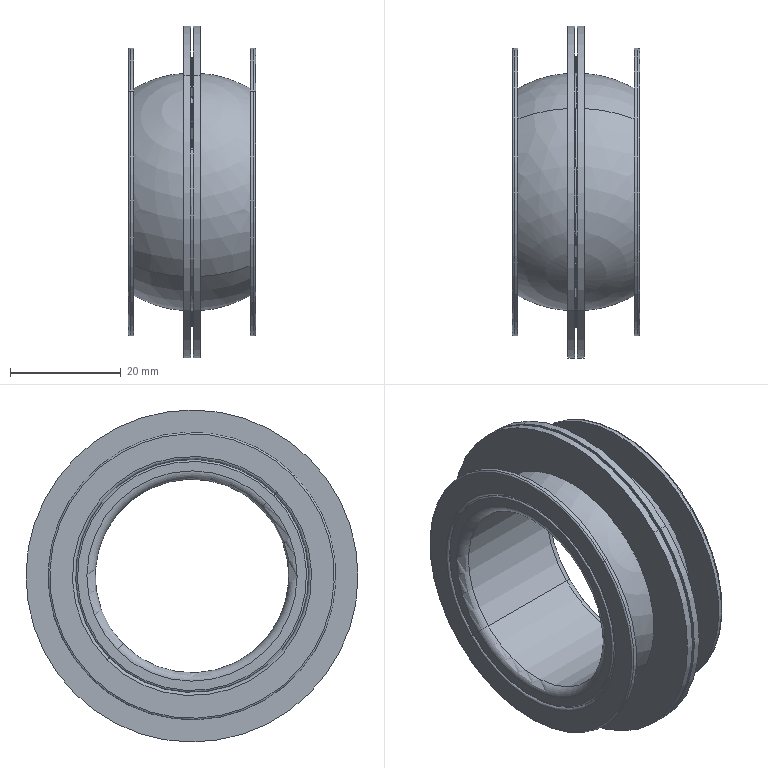Part | SolidWorks | features BaseBody 1 | 1 solid | 56 faces | volume 13898 mm3 | cylinder 18 | torus 16 | plane 12 | sphere 10 | commonest cylinder face diameters 42 x4 42.2 x4 52 x4 60 x4 35 x2
STEP:
#1=CARTESIAN_POINT('',(249.,13.531,-13.338));
#2=VERTEX_POINT('',#1);
#3=CARTESIAN_POINT('',(249.,-13.531,13.338));
#4=VERTEX_POINT('',#3);
#5=CARTESIAN_POINT('',(249.,0.,0.));
#6=DIRECTION('',(1.,0.,0.));
#7=DIRECTION('',(0.,-0.7122,0.702));
#8=AXIS2_PLACEMENT_3D('',#5,#6,#7);
#9=CIRCLE('',#8,19.);
#10=EDGE_CURVE('',#2,#4,#9,.T.);
#11=ORIENTED_EDGE('',*,*,#10,.F.);
#12=CARTESIAN_POINT('',(250.5,12.463,-12.285));
#13=VERTEX_POINT('',#12);
#14=CARTESIAN_POINT('',(250.5,13.531,-13.338));
#15=DIRECTION('',(0.,0.702,0.7122));
#16=DIRECTION('',(0.,-0.7122,0.702));
#17=AXIS2_PLACEMENT_3D('',#14,#15,#16);
#18=CIRCLE('',#17,1.5);
#19=EDGE_CURVE('',#2,#13,#18,.T.);
#20=ORIENTED_EDGE('',*,*,#19,.T.);
#21=CARTESIAN_POINT('',(250.5,-12.463,12.285));
#22=VERTEX_POINT('',#21);
#23=CARTESIAN_POINT('',(250.5,0.,0.));
#24=DIRECTION('',(-1.,0.,0.));
#25=DIRECTION('',(0.,-0.7122,0.702));
#26=AXIS2_PLACEMENT_3D('',#23,#24,#25);
#27=CIRCLE('',#26,17.5);
#28=EDGE_CURVE('',#22,#13,#27,.T.);
#29=ORIENTED_EDGE('',*,*,#28,.F.);
#30=CARTESIAN_POINT('',(250.5,-13.531,13.338));
#31=DIRECTION('',(0.,-0.702,-0.7122));
#32=DIRECTION('',(0.,0.7122,-0.702));
#33=AXIS2_PLACEMENT_3D('',#30,#31,#32);
#34=CIRCLE('',#33,1.5);
#35=EDGE_CURVE('',#4,#22,#34,.T.);
#36=ORIENTED_EDGE('',*,*,#35,.F.);
#37=EDGE_LOOP('',(#11,#20,#29,#36));
#38=FACE_OUTER_BOUND('',#37,.T.);
#39=CARTESIAN_POINT('',(250.5,0.,0.));
#40=DIRECTION('',(-1.,0.,0.));
#41=DIRECTION('',(0.,-0.7122,0.702));
#42=AXIS2_PLACEMENT_3D('',#39,#40,#41);
#43=TOROIDAL_SURFACE('',#42,19.,1.5);
#44=ADVANCED_FACE('',(#38),#43,.T.);
#45=CARTESIAN_POINT('',(272.,-13.531,13.338));
#46=VERTEX_POINT('',#45);
#47=CARTESIAN_POINT('',(272.,13.531,-13.338));
#48=VERTEX_POINT('',#47);
#49=CARTESIAN_POINT('',(272.,0.,0.));
#50=DIRECTION('',(-1.,0.,0.));
#51=DIRECTION('',(0.,0.7122,-0.702));
#52=AXIS2_PLACEMENT_3D('',#49,#50,#51);
#53=CIRCLE('',#52,19.);
#54=EDGE_CURVE('',#46,#48,#53,.T.);
#55=ORIENTED_EDGE('',*,*,#54,.F.);
#56=CARTESIAN_POINT('',(270.5,-12.463,12.285));
#57=VERTEX_POINT('',#56);
#58=CARTESIAN_POINT('',(270.5,-13.531,13.338));
#59=DIRECTION('',(0.,0.702,0.7122));
#60=DIRECTION('',(0.,-0.7122,0.702));
#61=AXIS2_PLACEMENT_3D('',#58,#59,#60);
#62=CIRCLE('',#61,1.5);
#63=EDGE_CURVE('',#46,#57,#62,.T.);
#64=ORIENTED_EDGE('',*,*,#63,.T.);
#65=CARTESIAN_POINT('',(270.5,12.463,-12.285));
#66=VERTEX_POINT('',#65);
#67=CARTESIAN_POINT('',(270.5,0.,0.));
#68=DIRECTION('',(1.,0.,0.));
#69=DIRECTION('',(0.,0.7122,-0.702));
#70=AXIS2_PLACEMENT_3D('',#67,#68,#69);
#71=CIRCLE('',#70,17.5);
#72=EDGE_CURVE('',#66,#57,#71,.T.);
#73=ORIENTED_EDGE('',*,*,#72,.F.);
#74=CARTESIAN_POINT('',(270.5,13.531,-13.338));
#75=DIRECTION('',(0.,-0.702,-0.7122));
#76=DIRECTION('',(0.,0.7122,-0.702));
#77=AXIS2_PLACEMENT_3D('',#74,#75,#76);
#78=CIRCLE('',#77,1.5);
#79=EDGE_CURVE('',#48,#66,#78,.T.);
#80=ORIENTED_EDGE('',*,*,#79,.F.);
#81=EDGE_LOOP('',(#55,#64,#73,#80));
#82=FACE_OUTER_BOUND('',#81,.T.);
#83=CARTESIAN_POINT('',(270.5,0.,0.));
#84=DIRECTION('',(1.,0.,0.));
#85=DIRECTION('',(0.,0.7122,-0.702));
#86=AXIS2_PLACEMENT_3D('',#83,#84,#85);
#87=TOROIDAL_SURFACE('',#86,19.,1.5);
#88=ADVANCED_FACE('',(#82),#87,.T.);
#89=CARTESIAN_POINT('',(260.25,15.092,15.31));
#90=VERTEX_POINT('',#89);
#91=CARTESIAN_POINT('',(260.25,-15.092,-15.31));
#92=VERTEX_POINT('',#91);
#93=CARTESIAN_POINT('',(260.25,0.,0.));
#94=DIRECTION('',(1.,0.,0.));
#95=DIRECTION('',(0.,0.7122,-0.702));
#96=AXIS2_PLACEMENT_3D('',#93,#94,#95);
#97=CIRCLE('',#96,21.499);
#98=EDGE_CURVE('',#90,#92,#97,.T.);
#99=ORIENTED_EDGE('',*,*,#98,.T.);
#100=CARTESIAN_POINT('',(260.75,-15.092,-15.31));
#101=VERTEX_POINT('',#100);
#102=CARTESIAN_POINT('',(260.5,0.,0.));
#103=DIRECTION('',(0.,-0.7122,0.702));
#104=DIRECTION('',(0.,-0.702,-0.7122));
#105=AXIS2_PLACEMENT_3D('',#102,#103,#104);
#106=CIRCLE('',#105,21.5);
#107=EDGE_CURVE('',#92,#101,#106,.T.);
#108=ORIENTED_EDGE('',*,*,#107,.T.);
#109=CARTESIAN_POINT('',(260.75,15.092,15.31));
#110=VERTEX_POINT('',#109);
#111=CARTESIAN_POINT('',(260.75,0.,0.));
#112=DIRECTION('',(1.,0.,0.));
#113=DIRECTION('',(0.,0.7122,-0.702));
#114=AXIS2_PLACEMENT_3D('',#111,#112,#113);
#115=CIRCLE('',#114,21.499);
#116=EDGE_CURVE('',#110,#101,#115,.T.);
#117=ORIENTED_EDGE('',*,*,#116,.F.);
#118=CARTESIAN_POINT('',(260.5,0.,0.));
#119=DIRECTION('',(0.,0.7122,-0.702));
#120=DIRECTION('',(0.,0.702,0.7122));
#121=AXIS2_PLACEMENT_3D('',#118,#119,#120);
#122=CIRCLE('',#121,21.5);
#123=EDGE_CURVE('',#90,#110,#122,.T.);
#124=ORIENTED_EDGE('',*,*,#123,.F.);
#125=EDGE_LOOP('',(#99,#108,#117,#124));
#126=FACE_OUTER_BOUND('',#125,.T.);
#127=CARTESIAN_POINT('',(260.5,0.,0.));
#128=DIRECTION('',(0.,-0.7122,0.702));
#129=DIRECTION('',(0.,0.702,0.7122));
#130=AXIS2_PLACEMENT_3D('',#127,#128,#129);
#131=SPHERICAL_SURFACE('',#130,21.5);
#132=ADVANCED_FACE('',(#126),#131,.T.);
#133=CARTESIAN_POINT('',(260.75,21.365,-21.061));
#134=VERTEX_POINT('',#133);
#135=CARTESIAN_POINT('',(260.75,-21.365,21.061));
#136=VERTEX_POINT('',#135);
#137=CARTESIAN_POINT('',(260.75,0.,0.));
#138=DIRECTION('',(1.,0.,0.));
#139=DIRECTION('',(0.,0.7122,-0.702));
#140=AXIS2_PLACEMENT_3D('',#137,#138,#139);
#141=CIRCLE('',#140,30.);
#142=EDGE_CURVE('',#134,#136,#141,.T.);
#143=ORIENTED_EDGE('',*,*,#142,.T.);
#144=CARTESIAN_POINT('',(262.,-21.365,21.061));
#145=VERTEX_POINT('',#144);
#146=CARTESIAN_POINT('',(260.5,-21.365,21.061));
#147=DIRECTION('',(1.,0.,0.));
#148=VECTOR('',#147,1000.);
#149=LINE('',#146,#148);
#150=EDGE_CURVE('',#136,#145,#149,.T.);
#151=ORIENTED_EDGE('',*,*,#150,.T.);
#152=CARTESIAN_POINT('',(262.,21.365,-21.061));
#153=VERTEX_POINT('',#152);
#154=CARTESIAN_POINT('',(262.,0.,0.));
#155=DIRECTION('',(1.,0.,0.));
#156=DIRECTION('',(0.,0.7122,-0.702));
#157=AXIS2_PLACEMENT_3D('',#154,#155,#156);
#158=CIRCLE('',#157,30.);
#159=EDGE_CURVE('',#153,#145,#158,.T.);
#160=ORIENTED_EDGE('',*,*,#159,.F.);
#161=CARTESIAN_POINT('',(260.5,21.365,-21.061));
#162=DIRECTION('',(1.,0.,0.));
#163=VECTOR('',#162,1000.);
#164=LINE('',#161,#163);
#165=EDGE_CURVE('',#134,#153,#164,.T.);
#166=ORIENTED_EDGE('',*,*,#165,.F.);
#167=EDGE_LOOP('',(#143,#151,#160,#166));
#168=FACE_OUTER_BOUND('',#167,.T.);
#169=CARTESIAN_POINT('',(260.5,0.,0.));
#170=DIRECTION('',(1.,0.,0.));
#171=DIRECTION('',(0.,0.7122,-0.702));
#172=AXIS2_PLACEMENT_3D('',#169,#170,#171);
#173=CYLINDRICAL_SURFACE('',#172,30.);
#174=ADVANCED_FACE('',(#168),#173,.T.);
#175=CARTESIAN_POINT('',(262.,15.057,15.274));
#176=VERTEX_POINT('',#175);
#177=CARTESIAN_POINT('',(262.,-15.057,-15.274));
#178=VERTEX_POINT('',#177);
#179=CARTESIAN_POINT('',(262.,0.,0.));
#180=DIRECTION('',(1.,0.,0.));
#181=DIRECTION('',(0.,0.7122,-0.702));
#182=AXIS2_PLACEMENT_3D('',#179,#180,#181);
#183=CIRCLE('',#182,21.448);
#184=EDGE_CURVE('',#176,#178,#183,.T.);
#185=ORIENTED_EDGE('',*,*,#184,.T.);
#186=CARTESIAN_POINT('',(271.,-13.171,-13.361));
#187=VERTEX_POINT('',#186);
#188=CARTESIAN_POINT('',(260.5,0.,0.));
#189=DIRECTION('',(0.,-0.7122,0.702));
#190=DIRECTION('',(0.,-0.702,-0.7122));
#191=AXIS2_PLACEMENT_3D('',#188,#189,#190);
#192=CIRCLE('',#191,21.5);
#193=EDGE_CURVE('',#178,#187,#192,.T.);
#194=ORIENTED_EDGE('',*,*,#193,.T.);
#195=CARTESIAN_POINT('',(271.,13.171,13.361));
#196=VERTEX_POINT('',#195);
#197=CARTESIAN_POINT('',(271.,0.,0.));
#198=DIRECTION('',(1.,0.,0.));
#199=DIRECTION('',(0.,0.7122,-0.702));
#200=AXIS2_PLACEMENT_3D('',#197,#198,#199);
#201=CIRCLE('',#200,18.762);
#202=EDGE_CURVE('',#196,#187,#201,.T.);
#203=ORIENTED_EDGE('',*,*,#202,.F.);
#204=CARTESIAN_POINT('',(260.5,0.,0.));
#205=DIRECTION('',(0.,0.7122,-0.702));
#206=DIRECTION('',(0.,0.702,0.7122));
#207=AXIS2_PLACEMENT_3D('',#204,#205,#206);
#208=CIRCLE('',#207,21.5);
#209=EDGE_CURVE('',#176,#196,#208,.T.);
#210=ORIENTED_EDGE('',*,*,#209,.F.);
#211=EDGE_LOOP('',(#185,#194,#203,#210));
#212=FACE_OUTER_BOUND('',#211,.T.);
#213=CARTESIAN_POINT('',(260.5,0.,0.));
#214=DIRECTION('',(0.,-0.7122,0.702));
#215=DIRECTION('',(0.,0.702,0.7122));
#216=AXIS2_PLACEMENT_3D('',#213,#214,#215);
#217=SPHERICAL_SURFACE('',#216,21.5);
#218=ADVANCED_FACE('',(#212),#217,.T.);
#219=CARTESIAN_POINT('',(271.,18.516,-18.253));
#220=VERTEX_POINT('',#219);
#221=CARTESIAN_POINT('',(271.,-18.516,18.253));
#222=VERTEX_POINT('',#221);
#223=CARTESIAN_POINT('',(271.,0.,0.));
#224=DIRECTION('',(1.,0.,0.));
#225=DIRECTION('',(0.,0.7122,-0.702));
#226=AXIS2_PLACEMENT_3D('',#223,#224,#225);
#227=CIRCLE('',#226,26.);
#228=EDGE_CURVE('',#220,#222,#227,.T.);
#229=ORIENTED_EDGE('',*,*,#228,.T.);
#230=CARTESIAN_POINT('',(271.7,-18.516,18.253));
#231=VERTEX_POINT('',#230);
#232=CARTESIAN_POINT('',(260.5,-18.516,18.253));
#233=DIRECTION('',(1.,0.,0.));
#234=VECTOR('',#233,1000.);
#235=LINE('',#232,#234);
#236=EDGE_CURVE('',#222,#231,#235,.T.);
#237=ORIENTED_EDGE('',*,*,#236,.T.);
#238=CARTESIAN_POINT('',(271.7,18.516,-18.253));
#239=VERTEX_POINT('',#238);
#240=CARTESIAN_POINT('',(271.7,0.,0.));
#241=DIRECTION('',(1.,0.,0.));
#242=DIRECTION('',(0.,0.7122,-0.702));
#243=AXIS2_PLACEMENT_3D('',#240,#241,#242);
#244=CIRCLE('',#243,26.);
#245=EDGE_CURVE('',#239,#231,#244,.T.);
#246=ORIENTED_EDGE('',*,*,#245,.F.);
#247=CARTESIAN_POINT('',(260.5,18.516,-18.253));
#248=DIRECTION('',(1.,0.,0.));
#249=VECTOR('',#248,1000.);
#250=LINE('',#247,#249);
#251=EDGE_CURVE('',#220,#239,#250,.T.);
#252=ORIENTED_EDGE('',*,*,#251,.F.);
#253=EDGE_LOOP('',(#229,#237,#246,#252));
#254=FACE_OUTER_BOUND('',#253,.T.);
#255=CARTESIAN_POINT('',(260.5,0.,0.));
#256=DIRECTION('',(1.,0.,0.));
#257=DIRECTION('',(0.,0.7122,-0.702));
#258=AXIS2_PLACEMENT_3D('',#255,#256,#257);
#259=CYLINDRICAL_SURFACE('',#258,26.);
#260=ADVANCED_FACE('',(#254),#259,.T.);
#261=ORIENTED_EDGE('',*,*,#245,.T.);
#262=CARTESIAN_POINT('',(272.,-18.302,18.042));
#263=VERTEX_POINT('',#262);
#264=CARTESIAN_POINT('',(271.7,-18.302,18.042));
#265=DIRECTION('',(0.,0.702,0.7122));
#266=DIRECTION('',(0.,-0.7122,0.702));
#267=AXIS2_PLACEMENT_3D('',#264,#265,#266);
#268=CIRCLE('',#267,0.3);
#269=EDGE_CURVE('',#231,#263,#268,.T.);
#270=ORIENTED_EDGE('',*,*,#269,.T.);
#271=CARTESIAN_POINT('',(272.,18.302,-18.042));
#272=VERTEX_POINT('',#271);
#273=CARTESIAN_POINT('',(272.,0.,0.));
#274=DIRECTION('',(1.,0.,0.));
#275=DIRECTION('',(0.,0.7122,-0.702));
#276=AXIS2_PLACEMENT_3D('',#273,#274,#275);
#277=CIRCLE('',#276,25.7);
#278=EDGE_CURVE('',#272,#263,#277,.T.);
#279=ORIENTED_EDGE('',*,*,#278,.F.);
#280=CARTESIAN_POINT('',(271.7,18.302,-18.042));
#281=DIRECTION('',(0.,-0.702,-0.7122));
#282=DIRECTION('',(0.,0.7122,-0.702));
#283=AXIS2_PLACEMENT_3D('',#280,#281,#282);
#284=CIRCLE('',#283,0.3);
#285=EDGE_CURVE('',#239,#272,#284,.T.);
#286=ORIENTED_EDGE('',*,*,#285,.F.);
#287=EDGE_LOOP('',(#261,#270,#279,#286));
#288=FACE_OUTER_BOUND('',#287,.T.);
#289=CARTESIAN_POINT('',(271.7,0.,0.));
#290=DIRECTION('',(1.,0.,0.));
#291=DIRECTION('',(0.,0.7122,-0.702));
#292=AXIS2_PLACEMENT_3D('',#289,#290,#291);
#293=TOROIDAL_SURFACE('',#292,25.7,0.3);
#294=ADVANCED_FACE('',(#288),#293,.T.);
#295=CARTESIAN_POINT('',(272.,15.383,-15.164));
#296=VERTEX_POINT('',#295);
#297=CARTESIAN_POINT('',(272.,-15.383,15.164));
#298=VERTEX_POINT('',#297);
#299=CARTESIAN_POINT('',(272.,0.,0.));
#300=DIRECTION('',(1.,0.,0.));
#301=DIRECTION('',(0.,0.7122,-0.702));
#302=AXIS2_PLACEMENT_3D('',#299,#300,#301);
#303=CIRCLE('',#302,21.6);
#304=EDGE_CURVE('',#296,#298,#303,.T.);
#305=ORIENTED_EDGE('',*,*,#304,.T.);
#306=CARTESIAN_POINT('',(271.5,-15.027,14.813));
#307=VERTEX_POINT('',#306);
#308=CARTESIAN_POINT('',(271.5,-15.383,15.164));
#309=DIRECTION('',(0.,0.702,0.7122));
#310=DIRECTION('',(0.,-0.7122,0.702));
#311=AXIS2_PLACEMENT_3D('',#308,#309,#310);
#312=CIRCLE('',#311,0.5);
#313=EDGE_CURVE('',#298,#307,#312,.T.);
#314=ORIENTED_EDGE('',*,*,#313,.T.);
#315=CARTESIAN_POINT('',(271.5,15.027,-14.813));
#316=VERTEX_POINT('',#315);
#317=CARTESIAN_POINT('',(271.5,0.,0.));
#318=DIRECTION('',(1.,0.,0.));
#319=DIRECTION('',(0.,0.7122,-0.702));
#320=AXIS2_PLACEMENT_3D('',#317,#318,#319);
#321=CIRCLE('',#320,21.1);
#322=EDGE_CURVE('',#316,#307,#321,.T.);
#323=ORIENTED_EDGE('',*,*,#322,.F.);
#324=CARTESIAN_POINT('',(271.5,15.383,-15.164));
#325=DIRECTION('',(0.,-0.702,-0.7122));
#326=DIRECTION('',(0.,0.7122,-0.702));
#327=AXIS2_PLACEMENT_3D('',#324,#325,#326);
#328=CIRCLE('',#327,0.5);
#329=EDGE_CURVE('',#296,#316,#328,.T.);
#330=ORIENTED_EDGE('',*,*,#329,.F.);
#331=EDGE_LOOP('',(#305,#314,#323,#330));
#332=FACE_OUTER_BOUND('',#331,.T.);
#333=CARTESIAN_POINT('',(271.5,0.,0.));
#334=DIRECTION('',(1.,0.,0.));
#335=DIRECTION('',(0.,0.7122,-0.702));
#336=AXIS2_PLACEMENT_3D('',#333,#334,#335);
#337=TOROIDAL_SURFACE('',#336,21.6,0.5);
#338=ADVANCED_FACE('',(#332),#337,.T.);
#339=CARTESIAN_POINT('',(271.2,-15.027,14.813));
#340=VERTEX_POINT('',#339);
#341=CARTESIAN_POINT('',(271.2,15.027,-14.813));
#342=VERTEX_POINT('',#341);
#343=CARTESIAN_POINT('',(271.2,0.,0.));
#344=DIRECTION('',(1.,0.,0.));
#345=DIRECTION('',(0.,0.7122,-0.702));
#346=AXIS2_PLACEMENT_3D('',#343,#344,#345);
#347=CIRCLE('',#346,21.1);
#348=EDGE_CURVE('',#340,#342,#347,.T.);
#349=ORIENTED_EDGE('',*,*,#348,.F.);
#350=CARTESIAN_POINT('',(260.5,-15.027,14.813));
#351=DIRECTION('',(1.,0.,0.));
#352=VECTOR('',#351,1000.);
#353=LINE('',#350,#352);
#354=EDGE_CURVE('',#340,#307,#353,.T.);
#355=ORIENTED_EDGE('',*,*,#354,.T.);
#356=CARTESIAN_POINT('',(271.5,0.,0.));
#357=DIRECTION('',(1.,0.,0.));
#358=DIRECTION('',(0.,0.7122,-0.702));
#359=AXIS2_PLACEMENT_3D('',#356,#357,#358);
#360=CIRCLE('',#359,21.1);
#361=EDGE_CURVE('',#307,#316,#360,.T.);
#362=ORIENTED_EDGE('',*,*,#361,.T.);
#363=CARTESIAN_POINT('',(260.5,15.027,-14.813));
#364=DIRECTION('',(1.,0.,0.));
#365=VECTOR('',#364,1000.);
#366=LINE('',#363,#365);
#367=EDGE_CURVE('',#342,#316,#366,.T.);
#368=ORIENTED_EDGE('',*,*,#367,.F.);
#369=EDGE_LOOP('',(#349,#355,#362,#368));
#370=FACE_OUTER_BOUND('',#369,.T.);
#371=CARTESIAN_POINT('',(260.5,0.,0.));
#372=DIRECTION('',(1.,0.,0.));
#373=DIRECTION('',(0.,0.7122,-0.702));
#374=AXIS2_PLACEMENT_3D('',#371,#372,#373);
#375=CYLINDRICAL_SURFACE('',#374,21.1);
#376=ADVANCED_FACE('',(#370),#375,.F.);
#377=CARTESIAN_POINT('',(271.2,14.955,-14.742));
#378=VERTEX_POINT('',#377);
#379=CARTESIAN_POINT('',(271.2,-14.955,14.742));
#380=VERTEX_POINT('',#379);
#381=CARTESIAN_POINT('',(271.2,0.,0.));
#382=DIRECTION('',(1.,0.,0.));
#383=DIRECTION('',(0.,0.7122,-0.702));
#384=AXIS2_PLACEMENT_3D('',#381,#382,#383);
#385=CIRCLE('',#384,21.);
#386=EDGE_CURVE('',#378,#380,#385,.T.);
#387=ORIENTED_EDGE('',*,*,#386,.T.);
#388=CARTESIAN_POINT('',(271.7,-14.955,14.742));
#389=VERTEX_POINT('',#388);
#390=CARTESIAN_POINT('',(260.5,-14.955,14.742));
#391=DIRECTION('',(1.,0.,0.));
#392=VECTOR('',#391,1000.);
#393=LINE('',#390,#392);
#394=EDGE_CURVE('',#380,#389,#393,.T.);
#395=ORIENTED_EDGE('',*,*,#394,.T.);
#396=CARTESIAN_POINT('',(271.7,14.955,-14.742));
#397=VERTEX_POINT('',#396);
#398=CARTESIAN_POINT('',(271.7,0.,0.));
#399=DIRECTION('',(1.,0.,0.));
#400=DIRECTION('',(0.,0.7122,-0.702));
#401=AXIS2_PLACEMENT_3D('',#398,#399,#400);
#402=CIRCLE('',#401,21.);
#403=EDGE_CURVE('',#397,#389,#402,.T.);
#404=ORIENTED_EDGE('',*,*,#403,.F.);
#405=CARTESIAN_POINT('',(260.5,14.955,-14.742));
#406=DIRECTION('',(1.,0.,0.));
#407=VECTOR('',#406,1000.);
#408=LINE('',#405,#407);
#409=EDGE_CURVE('',#378,#397,#408,.T.);
#410=ORIENTED_EDGE('',*,*,#409,.F.);
#411=EDGE_LOOP('',(#387,#395,#404,#410));
#412=FACE_OUTER_BOUND('',#411,.T.);
#413=CARTESIAN_POINT('',(260.5,0.,0.));
#414=DIRECTION('',(1.,0.,0.));
#415=DIRECTION('',(0.,0.7122,-0.702));
#416=AXIS2_PLACEMENT_3D('',#413,#414,#415);
#417=CYLINDRICAL_SURFACE('',#416,21.);
#418=ADVANCED_FACE('',(#412),#417,.T.);
#419=ORIENTED_EDGE('',*,*,#403,.T.);
#420=CARTESIAN_POINT('',(272.,-14.742,14.532));
#421=VERTEX_POINT('',#420);
#422=CARTESIAN_POINT('',(271.7,-14.742,14.532));
#423=DIRECTION('',(0.,0.702,0.7122));
#424=DIRECTION('',(0.,-0.7122,0.702));
#425=AXIS2_PLACEMENT_3D('',#422,#423,#424);
#426=CIRCLE('',#425,0.3);
#427=EDGE_CURVE('',#389,#421,#426,.T.);
#428=ORIENTED_EDGE('',*,*,#427,.T.);
#429=CARTESIAN_POINT('',(272.,14.742,-14.532));
#430=VERTEX_POINT('',#429);
#431=CARTESIAN_POINT('',(272.,0.,0.));
#432=DIRECTION('',(1.,0.,0.));
#433=DIRECTION('',(0.,0.7122,-0.702));
#434=AXIS2_PLACEMENT_3D('',#431,#432,#433);
#435=CIRCLE('',#434,20.7);
#436=EDGE_CURVE('',#430,#421,#435,.T.);
#437=ORIENTED_EDGE('',*,*,#436,.F.);
#438=CARTESIAN_POINT('',(271.7,14.742,-14.532));
#439=DIRECTION('',(0.,-0.702,-0.7122));
#440=DIRECTION('',(0.,0.7122,-0.702));
#441=AXIS2_PLACEMENT_3D('',#438,#439,#440);
#442=CIRCLE('',#441,0.3);
#443=EDGE_CURVE('',#397,#430,#442,.T.);
#444=ORIENTED_EDGE('',*,*,#443,.F.);
#445=EDGE_LOOP('',(#419,#428,#437,#444));
#446=FACE_OUTER_BOUND('',#445,.T.);
#447=CARTESIAN_POINT('',(271.7,0.,0.));
#448=DIRECTION('',(1.,0.,0.));
#449=DIRECTION('',(0.,0.7122,-0.702));
#450=AXIS2_PLACEMENT_3D('',#447,#448,#449);
#451=TOROIDAL_SURFACE('',#450,20.7,0.3);
#452=ADVANCED_FACE('',(#446),#451,.T.);
#453=CARTESIAN_POINT('',(250.5,0.,0.));
#454=DIRECTION('',(-1.,0.,0.));
#455=DIRECTION('',(0.,-0.7122,0.702));
#456=AXIS2_PLACEMENT_3D('',#453,#454,#455);
#457=CIRCLE('',#456,17.5);
#458=EDGE_CURVE('',#13,#22,#457,.T.);
#459=ORIENTED_EDGE('',*,*,#458,.T.);
#460=CARTESIAN_POINT('',(260.5,-12.463,12.285));
#461=DIRECTION('',(1.,0.,0.));
#462=VECTOR('',#461,1000.);
#463=LINE('',#460,#462);
#464=EDGE_CURVE('',#22,#57,#463,.T.);
#465=ORIENTED_EDGE('',*,*,#464,.T.);
#466=CARTESIAN_POINT('',(270.5,0.,0.));
#467=DIRECTION('',(1.,0.,0.));
#468=DIRECTION('',(0.,0.7122,-0.702));
#469=AXIS2_PLACEMENT_3D('',#466,#467,#468);
#470=CIRCLE('',#469,17.5);
#471=EDGE_CURVE('',#57,#66,#470,.T.);
#472=ORIENTED_EDGE('',*,*,#471,.T.);
#473=CARTESIAN_POINT('',(260.5,12.463,-12.285));
#474=DIRECTION('',(1.,0.,0.));
#475=VECTOR('',#474,1000.);
#476=LINE('',#473,#475);
#477=EDGE_CURVE('',#13,#66,#476,.T.);
#478=ORIENTED_EDGE('',*,*,#477,.F.);
#479=EDGE_LOOP('',(#459,#465,#472,#478));
#480=FACE_OUTER_BOUND('',#479,.T.);
#481=CARTESIAN_POINT('',(260.5,0.,0.));
#482=DIRECTION('',(1.,0.,0.));
#483=DIRECTION('',(0.,0.7122,-0.702));
#484=AXIS2_PLACEMENT_3D('',#481,#482,#483);
#485=CYLINDRICAL_SURFACE('',#484,17.5);
#486=ADVANCED_FACE('',(#480),#485,.F.);
#487=CARTESIAN_POINT('',(249.,14.742,-14.532));
#488=VERTEX_POINT('',#487);
#489=CARTESIAN_POINT('',(249.,-14.742,14.532));
#490=VERTEX_POINT('',#489);
#491=CARTESIAN_POINT('',(249.,0.,0.));
#492=DIRECTION('',(1.,0.,0.));
#493=DIRECTION('',(0.,0.7122,-0.702));
#494=AXIS2_PLACEMENT_3D('',#491,#492,#493);
#495=CIRCLE('',#494,20.7);
#496=EDGE_CURVE('',#488,#490,#495,.T.);
#497=ORIENTED_EDGE('',*,*,#496,.T.);
#498=CARTESIAN_POINT('',(249.3,-14.955,14.742));
#499=VERTEX_POINT('',#498);
#500=CARTESIAN_POINT('',(249.3,-14.742,14.532));
#501=DIRECTION('',(0.,0.702,0.7122));
#502=DIRECTION('',(0.,-0.7122,0.702));
#503=AXIS2_PLACEMENT_3D('',#500,#501,#502);
#504=CIRCLE('',#503,0.3);
#505=EDGE_CURVE('',#490,#499,#504,.T.);
#506=ORIENTED_EDGE('',*,*,#505,.T.);
#507=CARTESIAN_POINT('',(249.3,14.955,-14.742));
#508=VERTEX_POINT('',#507);
#509=CARTESIAN_POINT('',(249.3,0.,0.));
#510=DIRECTION('',(1.,0.,0.));
#511=DIRECTION('',(0.,0.7122,-0.702));
#512=AXIS2_PLACEMENT_3D('',#509,#510,#511);
#513=CIRCLE('',#512,21.);
#514=EDGE_CURVE('',#508,#499,#513,.T.);
#515=ORIENTED_EDGE('',*,*,#514,.F.);
#516=CARTESIAN_POINT('',(249.3,14.742,-14.532));
#517=DIRECTION('',(0.,-0.702,-0.7122));
#518=DIRECTION('',(0.,0.7122,-0.702));
#519=AXIS2_PLACEMENT_3D('',#516,#517,#518);
#520=CIRCLE('',#519,0.3);
#521=EDGE_CURVE('',#488,#508,#520,.T.);
#522=ORIENTED_EDGE('',*,*,#521,.F.);
#523=EDGE_LOOP('',(#497,#506,#515,#522));
#524=FACE_OUTER_BOUND('',#523,.T.);
#525=CARTESIAN_POINT('',(249.3,0.,0.));
#526=DIRECTION('',(1.,0.,0.));
#527=DIRECTION('',(0.,0.7122,-0.702));
#528=AXIS2_PLACEMENT_3D('',#525,#526,#527);
#529=TOROIDAL_SURFACE('',#528,20.7,0.3);
#530=ADVANCED_FACE('',(#524),#529,.T.);
#531=ORIENTED_EDGE('',*,*,#514,.T.);
#532=CARTESIAN_POINT('',(249.8,-14.955,14.742));
#533=VERTEX_POINT('',#532);
#534=CARTESIAN_POINT('',(260.5,-14.955,14.742));
#535=DIRECTION('',(1.,0.,0.));
#536=VECTOR('',#535,1000.);
#537=LINE('',#534,#536);
#538=EDGE_CURVE('',#499,#533,#537,.T.);
#539=ORIENTED_EDGE('',*,*,#538,.T.);
#540=CARTESIAN_POINT('',(249.8,14.955,-14.742));
#541=VERTEX_POINT('',#540);
#542=CARTESIAN_POINT('',(249.8,0.,0.));
#543=DIRECTION('',(1.,0.,0.));
#544=DIRECTION('',(0.,0.7122,-0.702));
#545=AXIS2_PLACEMENT_3D('',#542,#543,#544);
#546=CIRCLE('',#545,21.);
#547=EDGE_CURVE('',#541,#533,#546,.T.);
#548=ORIENTED_EDGE('',*,*,#547,.F.);
#549=CARTESIAN_POINT('',(260.5,14.955,-14.742));
#550=DIRECTION('',(1.,0.,0.));
#551=VECTOR('',#550,1000.);
#552=LINE('',#549,#551);
#553=EDGE_CURVE('',#508,#541,#552,.T.);
#554=ORIENTED_EDGE('',*,*,#553,.F.);
#555=EDGE_LOOP('',(#531,#539,#548,#554));
#556=FACE_OUTER_BOUND('',#555,.T.);
#557=CARTESIAN_POINT('',(260.5,0.,0.));
#558=DIRECTION('',(1.,0.,0.));
#559=DIRECTION('',(0.,0.7122,-0.702));
#560=AXIS2_PLACEMENT_3D('',#557,#558,#559);
#561=CYLINDRICAL_SURFACE('',#560,21.);
#562=ADVANCED_FACE('',(#556),#561,.T.);
#563=CARTESIAN_POINT('',(249.5,-15.027,14.813));
#564=VERTEX_POINT('',#563);
#565=CARTESIAN_POINT('',(249.5,15.027,-14.813));
#566=VERTEX_POINT('',#565);
#567=CARTESIAN_POINT('',(249.5,0.,0.));
#568=DIRECTION('',(1.,0.,0.));
#569=DIRECTION('',(0.,0.7122,-0.702));
#570=AXIS2_PLACEMENT_3D('',#567,#568,#569);
#571=CIRCLE('',#570,21.1);
#572=EDGE_CURVE('',#564,#566,#571,.T.);
#573=ORIENTED_EDGE('',*,*,#572,.F.);
#574=CARTESIAN_POINT('',(249.8,-15.027,14.813));
#575=VERTEX_POINT('',#574);
#576=CARTESIAN_POINT('',(260.5,-15.027,14.813));
#577=DIRECTION('',(1.,0.,0.));
#578=VECTOR('',#577,1000.);
#579=LINE('',#576,#578);
#580=EDGE_CURVE('',#564,#575,#579,.T.);
#581=ORIENTED_EDGE('',*,*,#580,.T.);
#582=CARTESIAN_POINT('',(249.8,15.027,-14.813));
#583=VERTEX_POINT('',#582);
#584=CARTESIAN_POINT('',(249.8,0.,0.));
#585=DIRECTION('',(1.,0.,0.));
#586=DIRECTION('',(0.,0.7122,-0.702));
#587=AXIS2_PLACEMENT_3D('',#584,#585,#586);
#588=CIRCLE('',#587,21.1);
#589=EDGE_CURVE('',#575,#583,#588,.T.);
#590=ORIENTED_EDGE('',*,*,#589,.T.);
#591=CARTESIAN_POINT('',(260.5,15.027,-14.813));
#592=DIRECTION('',(1.,0.,0.));
#593=VECTOR('',#592,1000.);
#594=LINE('',#591,#593);
#595=EDGE_CURVE('',#566,#583,#594,.T.);
#596=ORIENTED_EDGE('',*,*,#595,.F.);
#597=EDGE_LOOP('',(#573,#581,#590,#596));
#598=FACE_OUTER_BOUND('',#597,.T.);
#599=CARTESIAN_POINT('',(260.5,0.,0.));
#600=DIRECTION('',(1.,0.,0.));
#601=DIRECTION('',(0.,0.7122,-0.702));
#602=AXIS2_PLACEMENT_3D('',#599,#600,#601);
#603=CYLINDRICAL_SURFACE('',#602,21.1);
#604=ADVANCED_FACE('',(#598),#603,.F.);
#605=CARTESIAN_POINT('',(249.5,0.,0.));
#606=DIRECTION('',(1.,0.,0.));
#607=DIRECTION('',(0.,0.7122,-0.702));
#608=AXIS2_PLACEMENT_3D('',#605,#606,#607);
#609=CIRCLE('',#608,21.1);
#610=EDGE_CURVE('',#566,#564,#609,.T.);
#611=ORIENTED_EDGE('',*,*,#610,.T.);
#612=CARTESIAN_POINT('',(249.,-15.383,15.164));
#613=VERTEX_POINT('',#612);
#614=CARTESIAN_POINT('',(249.5,-15.383,15.164));
#615=DIRECTION('',(0.,0.702,0.7122));
#616=DIRECTION('',(0.,-0.7122,0.702));
#617=AXIS2_PLACEMENT_3D('',#614,#615,#616);
#618=CIRCLE('',#617,0.5);
#619=EDGE_CURVE('',#564,#613,#618,.T.);
#620=ORIENTED_EDGE('',*,*,#619,.T.);
#621=CARTESIAN_POINT('',(249.,15.383,-15.164));
#622=VERTEX_POINT('',#621);
#623=CARTESIAN_POINT('',(249.,0.,0.));
#624=DIRECTION('',(1.,0.,0.));
#625=DIRECTION('',(0.,0.7122,-0.702));
#626=AXIS2_PLACEMENT_3D('',#623,#624,#625);
#627=CIRCLE('',#626,21.6);
#628=EDGE_CURVE('',#622,#613,#627,.T.);
#629=ORIENTED_EDGE('',*,*,#628,.F.);
#630=CARTESIAN_POINT('',(249.5,15.383,-15.164));
#631=DIRECTION('',(0.,-0.702,-0.7122));
#632=DIRECTION('',(0.,0.7122,-0.702));
#633=AXIS2_PLACEMENT_3D('',#630,#631,#632);
#634=CIRCLE('',#633,0.5);
#635=EDGE_CURVE('',#566,#622,#634,.T.);
#636=ORIENTED_EDGE('',*,*,#635,.F.);
#637=EDGE_LOOP('',(#611,#620,#629,#636));
#638=FACE_OUTER_BOUND('',#637,.T.);
#639=CARTESIAN_POINT('',(249.5,0.,0.));
#640=DIRECTION('',(1.,0.,0.));
#641=DIRECTION('',(0.,0.7122,-0.702));
#642=AXIS2_PLACEMENT_3D('',#639,#640,#641);
#643=TOROIDAL_SURFACE('',#642,21.6,0.5);
#644=ADVANCED_FACE('',(#638),#643,.T.);
#645=CARTESIAN_POINT('',(249.,18.302,-18.042));
#646=VERTEX_POINT('',#645);
#647=CARTESIAN_POINT('',(249.,-18.302,18.042));
#648=VERTEX_POINT('',#647);
#649=CARTESIAN_POINT('',(249.,0.,0.));
#650=DIRECTION('',(1.,0.,0.));
#651=DIRECTION('',(0.,0.7122,-0.702));
#652=AXIS2_PLACEMENT_3D('',#649,#650,#651);
#653=CIRCLE('',#652,25.7);
#654=EDGE_CURVE('',#646,#648,#653,.T.);
#655=ORIENTED_EDGE('',*,*,#654,.T.);
#656=CARTESIAN_POINT('',(249.3,-18.516,18.253));
#657=VERTEX_POINT('',#656);
#658=CARTESIAN_POINT('',(249.3,-18.302,18.042));
#659=DIRECTION('',(0.,0.702,0.7122));
#660=DIRECTION('',(0.,-0.7122,0.702));
#661=AXIS2_PLACEMENT_3D('',#658,#659,#660);
#662=CIRCLE('',#661,0.3);
#663=EDGE_CURVE('',#648,#657,#662,.T.);
#664=ORIENTED_EDGE('',*,*,#663,.T.);
#665=CARTESIAN_POINT('',(249.3,18.516,-18.253));
#666=VERTEX_POINT('',#665);
#667=CARTESIAN_POINT('',(249.3,0.,0.));
#668=DIRECTION('',(1.,0.,0.));
#669=DIRECTION('',(0.,0.7122,-0.702));
#670=AXIS2_PLACEMENT_3D('',#667,#668,#669);
#671=CIRCLE('',#670,26.);
#672=EDGE_CURVE('',#666,#657,#671,.T.);
#673=ORIENTED_EDGE('',*,*,#672,.F.);
#674=CARTESIAN_POINT('',(249.3,18.302,-18.042));
#675=DIRECTION('',(0.,-0.702,-0.7122));
#676=DIRECTION('',(0.,0.7122,-0.702));
#677=AXIS2_PLACEMENT_3D('',#674,#675,#676);
#678=CIRCLE('',#677,0.3);
#679=EDGE_CURVE('',#646,#666,#678,.T.);
#680=ORIENTED_EDGE('',*,*,#679,.F.);
#681=EDGE_LOOP('',(#655,#664,#673,#680));
#682=FACE_OUTER_BOUND('',#681,.T.);
#683=CARTESIAN_POINT('',(249.3,0.,0.));
#684=DIRECTION('',(1.,0.,0.));
#685=DIRECTION('',(0.,0.7122,-0.702));
#686=AXIS2_PLACEMENT_3D('',#683,#684,#685);
#687=TOROIDAL_SURFACE('',#686,25.7,0.3);
#688=ADVANCED_FACE('',(#682),#687,.T.);
#689=ORIENTED_EDGE('',*,*,#672,.T.);
#690=CARTESIAN_POINT('',(250.,-18.516,18.253));
#691=VERTEX_POINT('',#690);
#692=CARTESIAN_POINT('',(260.5,-18.516,18.253));
#693=DIRECTION('',(1.,0.,0.));
#694=VECTOR('',#693,1000.);
#695=LINE('',#692,#694);
#696=EDGE_CURVE('',#657,#691,#695,.T.);
#697=ORIENTED_EDGE('',*,*,#696,.T.);
#698=CARTESIAN_POINT('',(250.,18.516,-18.253));
#699=VERTEX_POINT('',#698);
#700=CARTESIAN_POINT('',(250.,0.,0.));
#701=DIRECTION('',(1.,0.,0.));
#702=DIRECTION('',(0.,0.7122,-0.702));
#703=AXIS2_PLACEMENT_3D('',#700,#701,#702);
#704=CIRCLE('',#703,26.);
#705=EDGE_CURVE('',#699,#691,#704,.T.);
#706=ORIENTED_EDGE('',*,*,#705,.F.);
#707=CARTESIAN_POINT('',(260.5,18.516,-18.253));
#708=DIRECTION('',(1.,0.,0.));
#709=VECTOR('',#708,1000.);
#710=LINE('',#707,#709);
#711=EDGE_CURVE('',#666,#699,#710,.T.);
#712=ORIENTED_EDGE('',*,*,#711,.F.);
#713=EDGE_LOOP('',(#689,#697,#706,#712));
#714=FACE_OUTER_BOUND('',#713,.T.);
#715=CARTESIAN_POINT('',(260.5,0.,0.));
#716=DIRECTION('',(1.,0.,0.));
#717=DIRECTION('',(0.,0.7122,-0.702));
#718=AXIS2_PLACEMENT_3D('',#715,#716,#717);
#719=CYLINDRICAL_SURFACE('',#718,26.);
#720=ADVANCED_FACE('',(#714),#719,.T.);
#721=CARTESIAN_POINT('',(250.,13.171,13.361));
#722=VERTEX_POINT('',#721);
#723=CARTESIAN_POINT('',(250.,-13.171,-13.361));
#724=VERTEX_POINT('',#723);
#725=CARTESIAN_POINT('',(250.,0.,0.));
#726=DIRECTION('',(1.,0.,0.));
#727=DIRECTION('',(0.,0.7122,-0.702));
#728=AXIS2_PLACEMENT_3D('',#725,#726,#727);
#729=CIRCLE('',#728,18.762);
#730=EDGE_CURVE('',#722,#724,#729,.T.);
#731=ORIENTED_EDGE('',*,*,#730,.T.);
#732=CARTESIAN_POINT('',(259.,-15.057,-15.274));
#733=VERTEX_POINT('',#732);
#734=CARTESIAN_POINT('',(260.5,0.,0.));
#735=DIRECTION('',(0.,-0.7122,0.702));
#736=DIRECTION('',(0.,-0.702,-0.7122));
#737=AXIS2_PLACEMENT_3D('',#734,#735,#736);
#738=CIRCLE('',#737,21.5);
#739=EDGE_CURVE('',#724,#733,#738,.T.);
#740=ORIENTED_EDGE('',*,*,#739,.T.);
#741=CARTESIAN_POINT('',(259.,15.057,15.274));
#742=VERTEX_POINT('',#741);
#743=CARTESIAN_POINT('',(259.,0.,0.));
#744=DIRECTION('',(1.,0.,0.));
#745=DIRECTION('',(0.,0.7122,-0.702));
#746=AXIS2_PLACEMENT_3D('',#743,#744,#745);
#747=CIRCLE('',#746,21.448);
#748=EDGE_CURVE('',#742,#733,#747,.T.);
#749=ORIENTED_EDGE('',*,*,#748,.F.);
#750=CARTESIAN_POINT('',(260.5,0.,0.));
#751=DIRECTION('',(0.,0.7122,-0.702));
#752=DIRECTION('',(0.,0.702,0.7122));
#753=AXIS2_PLACEMENT_3D('',#750,#751,#752);
#754=CIRCLE('',#753,21.5);
#755=EDGE_CURVE('',#722,#742,#754,.T.);
#756=ORIENTED_EDGE('',*,*,#755,.F.);
#757=EDGE_LOOP('',(#731,#740,#749,#756));
#758=FACE_OUTER_BOUND('',#757,.T.);
#759=CARTESIAN_POINT('',(260.5,0.,0.));
#760=DIRECTION('',(0.,-0.7122,0.702));
#761=DIRECTION('',(0.,0.702,0.7122));
#762=AXIS2_PLACEMENT_3D('',#759,#760,#761);
#763=SPHERICAL_SURFACE('',#762,21.5);
#764=ADVANCED_FACE('',(#758),#763,.T.);
#765=CARTESIAN_POINT('',(259.,21.365,-21.061));
#766=VERTEX_POINT('',#765);
#767=CARTESIAN_POINT('',(259.,-21.365,21.061));
#768=VERTEX_POINT('',#767);
#769=CARTESIAN_POINT('',(259.,0.,0.));
#770=DIRECTION('',(1.,0.,0.));
#771=DIRECTION('',(0.,0.7122,-0.702));
#772=AXIS2_PLACEMENT_3D('',#769,#770,#771);
#773=CIRCLE('',#772,30.);
#774=EDGE_CURVE('',#766,#768,#773,.T.);
#775=ORIENTED_EDGE('',*,*,#774,.T.);
#776=CARTESIAN_POINT('',(260.25,-21.365,21.061));
#777=VERTEX_POINT('',#776);
#778=CARTESIAN_POINT('',(260.5,-21.365,21.061));
#779=DIRECTION('',(1.,0.,0.));
#780=VECTOR('',#779,1000.);
#781=LINE('',#778,#780);
#782=EDGE_CURVE('',#768,#777,#781,.T.);
#783=ORIENTED_EDGE('',*,*,#782,.T.);
#784=CARTESIAN_POINT('',(260.25,21.365,-21.061));
#785=VERTEX_POINT('',#784);
#786=CARTESIAN_POINT('',(260.25,0.,0.));
#787=DIRECTION('',(1.,0.,0.));
#788=DIRECTION('',(0.,0.7122,-0.702));
#789=AXIS2_PLACEMENT_3D('',#786,#787,#788);
#790=CIRCLE('',#789,30.);
#791=EDGE_CURVE('',#785,#777,#790,.T.);
#792=ORIENTED_EDGE('',*,*,#791,.F.);
#793=CARTESIAN_POINT('',(260.5,21.365,-21.061));
#794=DIRECTION('',(1.,0.,0.));
#795=VECTOR('',#794,1000.);
#796=LINE('',#793,#795);
#797=EDGE_CURVE('',#766,#785,#796,.T.);
#798=ORIENTED_EDGE('',*,*,#797,.F.);
#799=EDGE_LOOP('',(#775,#783,#792,#798));
#800=FACE_OUTER_BOUND('',#799,.T.);
#801=CARTESIAN_POINT('',(260.5,0.,0.));
#802=DIRECTION('',(1.,0.,0.));
#803=DIRECTION('',(0.,0.7122,-0.702));
#804=AXIS2_PLACEMENT_3D('',#801,#802,#803);
#805=CYLINDRICAL_SURFACE('',#804,30.);
#806=ADVANCED_FACE('',(#800),#805,.T.);
#807=ORIENTED_EDGE('',*,*,#791,.T.);
#808=CARTESIAN_POINT('',(260.25,0.,0.));
#809=DIRECTION('',(1.,0.,0.));
#810=DIRECTION('',(0.,0.7122,-0.702));
#811=AXIS2_PLACEMENT_3D('',#808,#809,#810);
#812=CIRCLE('',#811,30.);
#813=EDGE_CURVE('',#777,#785,#812,.T.);
#814=ORIENTED_EDGE('',*,*,#813,.T.);
#815=EDGE_LOOP('',(#807,#814));
#816=FACE_OUTER_BOUND('',#815,.T.);
#817=ORIENTED_EDGE('',*,*,#98,.F.);
#818=CARTESIAN_POINT('',(260.25,0.,0.));
#819=DIRECTION('',(1.,0.,0.));
#820=DIRECTION('',(0.,0.7122,-0.702));
#821=AXIS2_PLACEMENT_3D('',#818,#819,#820);
#822=CIRCLE('',#821,21.499);
#823=EDGE_CURVE('',#92,#90,#822,.T.);
#824=ORIENTED_EDGE('',*,*,#823,.F.);
#825=EDGE_LOOP('',(#817,#824));
#826=FACE_BOUND('',#825,.T.);
#827=CARTESIAN_POINT('',(260.25,21.061,21.365));
#828=DIRECTION('',(1.,0.,0.));
#829=DIRECTION('',(0.,0.7122,-0.702));
#830=AXIS2_PLACEMENT_3D('',#827,#828,#829);
#831=PLANE('',#830);
#832=ADVANCED_FACE('',(#816,#826),#831,.T.);
#833=ORIENTED_EDGE('',*,*,#782,.F.);
#834=CARTESIAN_POINT('',(259.,0.,0.));
#835=DIRECTION('',(1.,0.,0.));
#836=DIRECTION('',(0.,0.7122,-0.702));
#837=AXIS2_PLACEMENT_3D('',#834,#835,#836);
#838=CIRCLE('',#837,30.);
#839=EDGE_CURVE('',#768,#766,#838,.T.);
#840=ORIENTED_EDGE('',*,*,#839,.T.);
#841=ORIENTED_EDGE('',*,*,#797,.T.);
#842=ORIENTED_EDGE('',*,*,#813,.F.);
#843=EDGE_LOOP('',(#833,#840,#841,#842));
#844=FACE_OUTER_BOUND('',#843,.T.);
#845=CARTESIAN_POINT('',(260.5,0.,0.));
#846=DIRECTION('',(1.,0.,0.));
#847=DIRECTION('',(0.,0.7122,-0.702));
#848=AXIS2_PLACEMENT_3D('',#845,#846,#847);
#849=CYLINDRICAL_SURFACE('',#848,30.);
#850=ADVANCED_FACE('',(#844),#849,.T.);
#851=ORIENTED_EDGE('',*,*,#748,.T.);
#852=CARTESIAN_POINT('',(259.,0.,0.));
#853=DIRECTION('',(1.,0.,0.));
#854=DIRECTION('',(0.,0.7122,-0.702));
#855=AXIS2_PLACEMENT_3D('',#852,#853,#854);
#856=CIRCLE('',#855,21.448);
#857=EDGE_CURVE('',#733,#742,#856,.T.);
#858=ORIENTED_EDGE('',*,*,#857,.T.);
#859=EDGE_LOOP('',(#851,#858));
#860=FACE_BOUND('',#859,.T.);
#861=ORIENTED_EDGE('',*,*,#774,.F.);
#862=ORIENTED_EDGE('',*,*,#839,.F.);
#863=EDGE_LOOP('',(#861,#862));
#864=FACE_OUTER_BOUND('',#863,.T.);
#865=CARTESIAN_POINT('',(259.,15.057,15.274));
#866=DIRECTION('',(-1.,0.,0.));
#867=DIRECTION('',(0.,-0.7122,0.702));
#868=AXIS2_PLACEMENT_3D('',#865,#866,#867);
#869=PLANE('',#868);
#870=ADVANCED_FACE('',(#860,#864),#869,.T.);
#871=ORIENTED_EDGE('',*,*,#739,.F.);
#872=CARTESIAN_POINT('',(250.,0.,0.));
#873=DIRECTION('',(1.,0.,0.));
#874=DIRECTION('',(0.,0.7122,-0.702));
#875=AXIS2_PLACEMENT_3D('',#872,#873,#874);
#876=CIRCLE('',#875,18.762);
#877=EDGE_CURVE('',#724,#722,#876,.T.);
#878=ORIENTED_EDGE('',*,*,#877,.T.);
#879=ORIENTED_EDGE('',*,*,#755,.T.);
#880=ORIENTED_EDGE('',*,*,#857,.F.);
#881=EDGE_LOOP('',(#871,#878,#879,#880));
#882=FACE_OUTER_BOUND('',#881,.T.);
#883=CARTESIAN_POINT('',(260.5,0.,0.));
#884=DIRECTION('',(0.,-0.7122,0.702));
#885=DIRECTION('',(0.,0.702,0.7122));
#886=AXIS2_PLACEMENT_3D('',#883,#884,#885);
#887=SPHERICAL_SURFACE('',#886,21.5);
#888=ADVANCED_FACE('',(#882),#887,.T.);
#889=ORIENTED_EDGE('',*,*,#705,.T.);
#890=CARTESIAN_POINT('',(250.,0.,0.));
#891=DIRECTION('',(1.,0.,0.));
#892=DIRECTION('',(0.,0.7122,-0.702));
#893=AXIS2_PLACEMENT_3D('',#890,#891,#892);
#894=CIRCLE('',#893,26.);
#895=EDGE_CURVE('',#691,#699,#894,.T.);
#896=ORIENTED_EDGE('',*,*,#895,.T.);
#897=EDGE_LOOP('',(#889,#896));
#898=FACE_OUTER_BOUND('',#897,.T.);
#899=ORIENTED_EDGE('',*,*,#730,.F.);
#900=ORIENTED_EDGE('',*,*,#877,.F.);
#901=EDGE_LOOP('',(#899,#900));
#902=FACE_BOUND('',#901,.T.);
#903=CARTESIAN_POINT('',(250.,18.253,18.516));
#904=DIRECTION('',(1.,0.,0.));
#905=DIRECTION('',(0.,0.7122,-0.702));
#906=AXIS2_PLACEMENT_3D('',#903,#904,#905);
#907=PLANE('',#906);
#908=ADVANCED_FACE('',(#898,#902),#907,.T.);
#909=ORIENTED_EDGE('',*,*,#696,.F.);
#910=CARTESIAN_POINT('',(249.3,0.,0.));
#911=DIRECTION('',(1.,0.,0.));
#912=DIRECTION('',(0.,0.7122,-0.702));
#913=AXIS2_PLACEMENT_3D('',#910,#911,#912);
#914=CIRCLE('',#913,26.);
#915=EDGE_CURVE('',#657,#666,#914,.T.);
#916=ORIENTED_EDGE('',*,*,#915,.T.);
#917=ORIENTED_EDGE('',*,*,#711,.T.);
#918=ORIENTED_EDGE('',*,*,#895,.F.);
#919=EDGE_LOOP('',(#909,#916,#917,#918));
#920=FACE_OUTER_BOUND('',#919,.T.);
#921=CARTESIAN_POINT('',(260.5,0.,0.));
#922=DIRECTION('',(1.,0.,0.));
#923=DIRECTION('',(0.,0.7122,-0.702));
#924=AXIS2_PLACEMENT_3D('',#921,#922,#923);
#925=CYLINDRICAL_SURFACE('',#924,26.);
#926=ADVANCED_FACE('',(#920),#925,.T.);
#927=ORIENTED_EDGE('',*,*,#663,.F.);
#928=CARTESIAN_POINT('',(249.,0.,0.));
#929=DIRECTION('',(1.,0.,0.));
#930=DIRECTION('',(0.,0.7122,-0.702));
#931=AXIS2_PLACEMENT_3D('',#928,#929,#930);
#932=CIRCLE('',#931,25.7);
#933=EDGE_CURVE('',#648,#646,#932,.T.);
#934=ORIENTED_EDGE('',*,*,#933,.T.);
#935=ORIENTED_EDGE('',*,*,#679,.T.);
#936=ORIENTED_EDGE('',*,*,#915,.F.);
#937=EDGE_LOOP('',(#927,#934,#935,#936));
#938=FACE_OUTER_BOUND('',#937,.T.);
#939=CARTESIAN_POINT('',(249.3,0.,0.));
#940=DIRECTION('',(1.,0.,0.));
#941=DIRECTION('',(0.,0.7122,-0.702));
#942=AXIS2_PLACEMENT_3D('',#939,#940,#941);
#943=TOROIDAL_SURFACE('',#942,25.7,0.3);
#944=ADVANCED_FACE('',(#938),#943,.T.);
#945=ORIENTED_EDGE('',*,*,#628,.T.);
#946=CARTESIAN_POINT('',(249.,0.,0.));
#947=DIRECTION('',(1.,0.,0.));
#948=DIRECTION('',(0.,0.7122,-0.702));
#949=AXIS2_PLACEMENT_3D('',#946,#947,#948);
#950=CIRCLE('',#949,21.6);
#951=EDGE_CURVE('',#613,#622,#950,.T.);
#952=ORIENTED_EDGE('',*,*,#951,.T.);
#953=EDGE_LOOP('',(#945,#952));
#954=FACE_BOUND('',#953,.T.);
#955=ORIENTED_EDGE('',*,*,#654,.F.);
#956=ORIENTED_EDGE('',*,*,#933,.F.);
#957=EDGE_LOOP('',(#955,#956));
#958=FACE_OUTER_BOUND('',#957,.T.);
#959=CARTESIAN_POINT('',(249.,15.164,15.383));
#960=DIRECTION('',(-1.,0.,0.));
#961=DIRECTION('',(0.,-0.7122,0.702));
#962=AXIS2_PLACEMENT_3D('',#959,#960,#961);
#963=PLANE('',#962);
#964=ADVANCED_FACE('',(#954,#958),#963,.T.);
#965=ORIENTED_EDGE('',*,*,#619,.F.);
#966=ORIENTED_EDGE('',*,*,#572,.T.);
#967=ORIENTED_EDGE('',*,*,#635,.T.);
#968=ORIENTED_EDGE('',*,*,#951,.F.);
#969=EDGE_LOOP('',(#965,#966,#967,#968));
#970=FACE_OUTER_BOUND('',#969,.T.);
#971=CARTESIAN_POINT('',(249.5,0.,0.));
#972=DIRECTION('',(1.,0.,0.));
#973=DIRECTION('',(0.,0.7122,-0.702));
#974=AXIS2_PLACEMENT_3D('',#971,#972,#973);
#975=TOROIDAL_SURFACE('',#974,21.6,0.5);
#976=ADVANCED_FACE('',(#970),#975,.T.);
#977=ORIENTED_EDGE('',*,*,#580,.F.);
#978=ORIENTED_EDGE('',*,*,#610,.F.);
#979=ORIENTED_EDGE('',*,*,#595,.T.);
#980=CARTESIAN_POINT('',(249.8,0.,0.));
#981=DIRECTION('',(1.,0.,0.));
#982=DIRECTION('',(0.,0.7122,-0.702));
#983=AXIS2_PLACEMENT_3D('',#980,#981,#982);
#984=CIRCLE('',#983,21.1);
#985=EDGE_CURVE('',#583,#575,#984,.T.);
#986=ORIENTED_EDGE('',*,*,#985,.T.);
#987=EDGE_LOOP('',(#977,#978,#979,#986));
#988=FACE_OUTER_BOUND('',#987,.T.);
#989=CARTESIAN_POINT('',(260.5,0.,0.));
#990=DIRECTION('',(1.,0.,0.));
#991=DIRECTION('',(0.,0.7122,-0.702));
#992=AXIS2_PLACEMENT_3D('',#989,#990,#991);
#993=CYLINDRICAL_SURFACE('',#992,21.1);
#994=ADVANCED_FACE('',(#988),#993,.F.);
#995=ORIENTED_EDGE('',*,*,#547,.T.);
#996=CARTESIAN_POINT('',(249.8,0.,0.));
#997=DIRECTION('',(1.,0.,0.));
#998=DIRECTION('',(0.,0.7122,-0.702));
#999=AXIS2_PLACEMENT_3D('',#996,#997,#998);
#1000=CIRCLE('',#999,21.);
#1001=EDGE_CURVE('',#533,#541,#1000,.T.);
#1002=ORIENTED_EDGE('',*,*,#1001,.T.);
#1003=EDGE_LOOP('',(#995,#1002));
#1004=FACE_BOUND('',#1003,.T.);
#1005=ORIENTED_EDGE('',*,*,#985,.F.);
#1006=ORIENTED_EDGE('',*,*,#589,.F.);
#1007=EDGE_LOOP('',(#1005,#1006));
#1008=FACE_OUTER_BOUND('',#1007,.T.);
#1009=CARTESIAN_POINT('',(249.8,14.742,14.955));
#1010=DIRECTION('',(-1.,0.,0.));
#1011=DIRECTION('',(0.,-0.7122,0.702));
#1012=AXIS2_PLACEMENT_3D('',#1009,#1010,#1011);
#1013=PLANE('',#1012);
#1014=ADVANCED_FACE('',(#1004,#1008),#1013,.T.);
#1015=ORIENTED_EDGE('',*,*,#538,.F.);
#1016=CARTESIAN_POINT('',(249.3,0.,0.));
#1017=DIRECTION('',(1.,0.,0.));
#1018=DIRECTION('',(0.,0.7122,-0.702));
#1019=AXIS2_PLACEMENT_3D('',#1016,#1017,#1018);
#1020=CIRCLE('',#1019,21.);
#1021=EDGE_CURVE('',#499,#508,#1020,.T.);
#1022=ORIENTED_EDGE('',*,*,#1021,.T.);
#1023=ORIENTED_EDGE('',*,*,#553,.T.);
#1024=ORIENTED_EDGE('',*,*,#1001,.F.);
#1025=EDGE_LOOP('',(#1015,#1022,#1023,#1024));
#1026=FACE_OUTER_BOUND('',#1025,.T.);
#1027=CARTESIAN_POINT('',(260.5,0.,0.));
#1028=DIRECTION('',(1.,0.,0.));
#1029=DIRECTION('',(0.,0.7122,-0.702));
#1030=AXIS2_PLACEMENT_3D('',#1027,#1028,#1029);
#1031=CYLINDRICAL_SURFACE('',#1030,21.);
#1032=ADVANCED_FACE('',(#1026),#1031,.T.);
#1033=ORIENTED_EDGE('',*,*,#505,.F.);
#1034=CARTESIAN_POINT('',(249.,0.,0.));
#1035=DIRECTION('',(1.,0.,0.));
#1036=DIRECTION('',(0.,0.7122,-0.702));
#1037=AXIS2_PLACEMENT_3D('',#1034,#1035,#1036);
#1038=CIRCLE('',#1037,20.7);
#1039=EDGE_CURVE('',#490,#488,#1038,.T.);
#1040=ORIENTED_EDGE('',*,*,#1039,.T.);
#1041=ORIENTED_EDGE('',*,*,#521,.T.);
#1042=ORIENTED_EDGE('',*,*,#1021,.F.);
#1043=EDGE_LOOP('',(#1033,#1040,#1041,#1042));
#1044=FACE_OUTER_BOUND('',#1043,.T.);
#1045=CARTESIAN_POINT('',(249.3,0.,0.));
#1046=DIRECTION('',(1.,0.,0.));
#1047=DIRECTION('',(0.,0.7122,-0.702));
#1048=AXIS2_PLACEMENT_3D('',#1045,#1046,#1047);
#1049=TOROIDAL_SURFACE('',#1048,20.7,0.3);
#1050=ADVANCED_FACE('',(#1044),#1049,.T.);
#1051=CARTESIAN_POINT('',(249.,0.,0.));
#1052=DIRECTION('',(1.,0.,0.));
#1053=DIRECTION('',(0.,-0.7122,0.702));
#1054=AXIS2_PLACEMENT_3D('',#1051,#1052,#1053);
#1055=CIRCLE('',#1054,19.);
#1056=EDGE_CURVE('',#4,#2,#1055,.T.);
#1057=ORIENTED_EDGE('',*,*,#1056,.T.);
#1058=ORIENTED_EDGE('',*,*,#10,.T.);
#1059=EDGE_LOOP('',(#1057,#1058));
#1060=FACE_BOUND('',#1059,.T.);
#1061=ORIENTED_EDGE('',*,*,#496,.F.);
#1062=ORIENTED_EDGE('',*,*,#1039,.F.);
#1063=EDGE_LOOP('',(#1061,#1062));
#1064=FACE_OUTER_BOUND('',#1063,.T.);
#1065=CARTESIAN_POINT('',(249.,12.285,12.463));
#1066=DIRECTION('',(-1.,0.,0.));
#1067=DIRECTION('',(0.,-0.7122,0.702));
#1068=AXIS2_PLACEMENT_3D('',#1065,#1066,#1067);
#1069=PLANE('',#1068);
#1070=ADVANCED_FACE('',(#1060,#1064),#1069,.T.);
#1071=ORIENTED_EDGE('',*,*,#464,.F.);
#1072=ORIENTED_EDGE('',*,*,#28,.T.);
#1073=ORIENTED_EDGE('',*,*,#477,.T.);
#1074=ORIENTED_EDGE('',*,*,#72,.T.);
#1075=EDGE_LOOP('',(#1071,#1072,#1073,#1074));
#1076=FACE_OUTER_BOUND('',#1075,.T.);
#1077=CARTESIAN_POINT('',(260.5,0.,0.));
#1078=DIRECTION('',(1.,0.,0.));
#1079=DIRECTION('',(0.,0.7122,-0.702));
#1080=AXIS2_PLACEMENT_3D('',#1077,#1078,#1079);
#1081=CYLINDRICAL_SURFACE('',#1080,17.5);
#1082=ADVANCED_FACE('',(#1076),#1081,.F.);
#1083=CARTESIAN_POINT('',(272.,0.,0.));
#1084=DIRECTION('',(-1.,0.,0.));
#1085=DIRECTION('',(0.,0.7122,-0.702));
#1086=AXIS2_PLACEMENT_3D('',#1083,#1084,#1085);
#1087=CIRCLE('',#1086,19.);
#1088=EDGE_CURVE('',#48,#46,#1087,.T.);
#1089=ORIENTED_EDGE('',*,*,#1088,.T.);
#1090=ORIENTED_EDGE('',*,*,#54,.T.);
#1091=EDGE_LOOP('',(#1089,#1090));
#1092=FACE_BOUND('',#1091,.T.);
#1093=ORIENTED_EDGE('',*,*,#436,.T.);
#1094=CARTESIAN_POINT('',(272.,0.,0.));
#1095=DIRECTION('',(1.,0.,0.));
#1096=DIRECTION('',(0.,0.7122,-0.702));
#1097=AXIS2_PLACEMENT_3D('',#1094,#1095,#1096);
#1098=CIRCLE('',#1097,20.7);
#1099=EDGE_CURVE('',#421,#430,#1098,.T.);
#1100=ORIENTED_EDGE('',*,*,#1099,.T.);
#1101=EDGE_LOOP('',(#1093,#1100));
#1102=FACE_OUTER_BOUND('',#1101,.T.);
#1103=CARTESIAN_POINT('',(272.,12.285,12.463));
#1104=DIRECTION('',(1.,0.,0.));
#1105=DIRECTION('',(0.,0.7122,-0.702));
#1106=AXIS2_PLACEMENT_3D('',#1103,#1104,#1105);
#1107=PLANE('',#1106);
#1108=ADVANCED_FACE('',(#1092,#1102),#1107,.T.);
#1109=ORIENTED_EDGE('',*,*,#427,.F.);
#1110=CARTESIAN_POINT('',(271.7,0.,0.));
#1111=DIRECTION('',(1.,0.,0.));
#1112=DIRECTION('',(0.,0.7122,-0.702));
#1113=AXIS2_PLACEMENT_3D('',#1110,#1111,#1112);
#1114=CIRCLE('',#1113,21.);
#1115=EDGE_CURVE('',#389,#397,#1114,.T.);
#1116=ORIENTED_EDGE('',*,*,#1115,.T.);
#1117=ORIENTED_EDGE('',*,*,#443,.T.);
#1118=ORIENTED_EDGE('',*,*,#1099,.F.);
#1119=EDGE_LOOP('',(#1109,#1116,#1117,#1118));
#1120=FACE_OUTER_BOUND('',#1119,.T.);
#1121=CARTESIAN_POINT('',(271.7,0.,0.));
#1122=DIRECTION('',(1.,0.,0.));
#1123=DIRECTION('',(0.,0.7122,-0.702));
#1124=AXIS2_PLACEMENT_3D('',#1121,#1122,#1123);
#1125=TOROIDAL_SURFACE('',#1124,20.7,0.3);
#1126=ADVANCED_FACE('',(#1120),#1125,.T.);
#1127=ORIENTED_EDGE('',*,*,#394,.F.);
#1128=CARTESIAN_POINT('',(271.2,0.,0.));
#1129=DIRECTION('',(1.,0.,0.));
#1130=DIRECTION('',(0.,0.7122,-0.702));
#1131=AXIS2_PLACEMENT_3D('',#1128,#1129,#1130);
#1132=CIRCLE('',#1131,21.);
#1133=EDGE_CURVE('',#380,#378,#1132,.T.);
#1134=ORIENTED_EDGE('',*,*,#1133,.T.);
#1135=ORIENTED_EDGE('',*,*,#409,.T.);
#1136=ORIENTED_EDGE('',*,*,#1115,.F.);
#1137=EDGE_LOOP('',(#1127,#1134,#1135,#1136));
#1138=FACE_OUTER_BOUND('',#1137,.T.);
#1139=CARTESIAN_POINT('',(260.5,0.,0.));
#1140=DIRECTION('',(1.,0.,0.));
#1141=DIRECTION('',(0.,0.7122,-0.702));
#1142=AXIS2_PLACEMENT_3D('',#1139,#1140,#1141);
#1143=CYLINDRICAL_SURFACE('',#1142,21.);
#1144=ADVANCED_FACE('',(#1138),#1143,.T.);
#1145=CARTESIAN_POINT('',(271.2,0.,0.));
#1146=DIRECTION('',(1.,0.,0.));
#1147=DIRECTION('',(0.,0.7122,-0.702));
#1148=AXIS2_PLACEMENT_3D('',#1145,#1146,#1147);
#1149=CIRCLE('',#1148,21.1);
#1150=EDGE_CURVE('',#342,#340,#1149,.T.);
#1151=ORIENTED_EDGE('',*,*,#1150,.T.);
#1152=ORIENTED_EDGE('',*,*,#348,.T.);
#1153=EDGE_LOOP('',(#1151,#1152));
#1154=FACE_OUTER_BOUND('',#1153,.T.);
#1155=ORIENTED_EDGE('',*,*,#386,.F.);
#1156=ORIENTED_EDGE('',*,*,#1133,.F.);
#1157=EDGE_LOOP('',(#1155,#1156));
#1158=FACE_BOUND('',#1157,.T.);
#1159=CARTESIAN_POINT('',(271.2,14.742,14.955));
#1160=DIRECTION('',(1.,0.,0.));
#1161=DIRECTION('',(0.,0.7122,-0.702));
#1162=AXIS2_PLACEMENT_3D('',#1159,#1160,#1161);
#1163=PLANE('',#1162);
#1164=ADVANCED_FACE('',(#1154,#1158),#1163,.T.);
#1165=ORIENTED_EDGE('',*,*,#354,.F.);
#1166=ORIENTED_EDGE('',*,*,#1150,.F.);
#1167=ORIENTED_EDGE('',*,*,#367,.T.);
#1168=ORIENTED_EDGE('',*,*,#322,.T.);
#1169=EDGE_LOOP('',(#1165,#1166,#1167,#1168));
#1170=FACE_OUTER_BOUND('',#1169,.T.);
#1171=CARTESIAN_POINT('',(260.5,0.,0.));
#1172=DIRECTION('',(1.,0.,0.));
#1173=DIRECTION('',(0.,0.7122,-0.702));
#1174=AXIS2_PLACEMENT_3D('',#1171,#1172,#1173);
#1175=CYLINDRICAL_SURFACE('',#1174,21.1);
#1176=ADVANCED_FACE('',(#1170),#1175,.F.);
#1177=ORIENTED_EDGE('',*,*,#313,.F.);
#1178=CARTESIAN_POINT('',(272.,0.,0.));
#1179=DIRECTION('',(1.,0.,0.));
#1180=DIRECTION('',(0.,0.7122,-0.702));
#1181=AXIS2_PLACEMENT_3D('',#1178,#1179,#1180);
#1182=CIRCLE('',#1181,21.6);
#1183=EDGE_CURVE('',#298,#296,#1182,.T.);
#1184=ORIENTED_EDGE('',*,*,#1183,.T.);
#1185=ORIENTED_EDGE('',*,*,#329,.T.);
#1186=ORIENTED_EDGE('',*,*,#361,.F.);
#1187=EDGE_LOOP('',(#1177,#1184,#1185,#1186));
#1188=FACE_OUTER_BOUND('',#1187,.T.);
#1189=CARTESIAN_POINT('',(271.5,0.,0.));
#1190=DIRECTION('',(1.,0.,0.));
#1191=DIRECTION('',(0.,0.7122,-0.702));
#1192=AXIS2_PLACEMENT_3D('',#1189,#1190,#1191);
#1193=TOROIDAL_SURFACE('',#1192,21.6,0.5);
#1194=ADVANCED_FACE('',(#1188),#1193,.T.);
#1195=ORIENTED_EDGE('',*,*,#278,.T.);
#1196=CARTESIAN_POINT('',(272.,0.,0.));
#1197=DIRECTION('',(1.,0.,0.));
#1198=DIRECTION('',(0.,0.7122,-0.702));
#1199=AXIS2_PLACEMENT_3D('',#1196,#1197,#1198);
#1200=CIRCLE('',#1199,25.7);
#1201=EDGE_CURVE('',#263,#272,#1200,.T.);
#1202=ORIENTED_EDGE('',*,*,#1201,.T.);
#1203=EDGE_LOOP('',(#1195,#1202));
#1204=FACE_OUTER_BOUND('',#1203,.T.);
#1205=ORIENTED_EDGE('',*,*,#304,.F.);
#1206=ORIENTED_EDGE('',*,*,#1183,.F.);
#1207=EDGE_LOOP('',(#1205,#1206));
#1208=FACE_BOUND('',#1207,.T.);
#1209=CARTESIAN_POINT('',(272.,15.164,15.383));
#1210=DIRECTION('',(1.,0.,0.));
#1211=DIRECTION('',(0.,0.7122,-0.702));
#1212=AXIS2_PLACEMENT_3D('',#1209,#1210,#1211);
#1213=PLANE('',#1212);
#1214=ADVANCED_FACE('',(#1204,#1208),#1213,.T.);
#1215=ORIENTED_EDGE('',*,*,#269,.F.);
#1216=CARTESIAN_POINT('',(271.7,0.,0.));
#1217=DIRECTION('',(1.,0.,0.));
#1218=DIRECTION('',(0.,0.7122,-0.702));
#1219=AXIS2_PLACEMENT_3D('',#1216,#1217,#1218);
#1220=CIRCLE('',#1219,26.);
#1221=EDGE_CURVE('',#231,#239,#1220,.T.);
#1222=ORIENTED_EDGE('',*,*,#1221,.T.);
#1223=ORIENTED_EDGE('',*,*,#285,.T.);
#1224=ORIENTED_EDGE('',*,*,#1201,.F.);
#1225=EDGE_LOOP('',(#1215,#1222,#1223,#1224));
#1226=FACE_OUTER_BOUND('',#1225,.T.);
#1227=CARTESIAN_POINT('',(271.7,0.,0.));
#1228=DIRECTION('',(1.,0.,0.));
#1229=DIRECTION('',(0.,0.7122,-0.702));
#1230=AXIS2_PLACEMENT_3D('',#1227,#1228,#1229);
#1231=TOROIDAL_SURFACE('',#1230,25.7,0.3);
#1232=ADVANCED_FACE('',(#1226),#1231,.T.);
#1233=ORIENTED_EDGE('',*,*,#236,.F.);
#1234=CARTESIAN_POINT('',(271.,0.,0.));
#1235=DIRECTION('',(1.,0.,0.));
#1236=DIRECTION('',(0.,0.7122,-0.702));
#1237=AXIS2_PLACEMENT_3D('',#1234,#1235,#1236);
#1238=CIRCLE('',#1237,26.);
#1239=EDGE_CURVE('',#222,#220,#1238,.T.);
#1240=ORIENTED_EDGE('',*,*,#1239,.T.);
#1241=ORIENTED_EDGE('',*,*,#251,.T.);
#1242=ORIENTED_EDGE('',*,*,#1221,.F.);
#1243=EDGE_LOOP('',(#1233,#1240,#1241,#1242));
#1244=FACE_OUTER_BOUND('',#1243,.T.);
#1245=CARTESIAN_POINT('',(260.5,0.,0.));
#1246=DIRECTION('',(1.,0.,0.));
#1247=DIRECTION('',(0.,0.7122,-0.702));
#1248=AXIS2_PLACEMENT_3D('',#1245,#1246,#1247);
#1249=CYLINDRICAL_SURFACE('',#1248,26.);
#1250=ADVANCED_FACE('',(#1244),#1249,.T.);
#1251=ORIENTED_EDGE('',*,*,#202,.T.);
#1252=CARTESIAN_POINT('',(271.,0.,0.));
#1253=DIRECTION('',(1.,0.,0.));
#1254=DIRECTION('',(0.,0.7122,-0.702));
#1255=AXIS2_PLACEMENT_3D('',#1252,#1253,#1254);
#1256=CIRCLE('',#1255,18.762);
#1257=EDGE_CURVE('',#187,#196,#1256,.T.);
#1258=ORIENTED_EDGE('',*,*,#1257,.T.);
#1259=EDGE_LOOP('',(#1251,#1258));
#1260=FACE_BOUND('',#1259,.T.);
#1261=ORIENTED_EDGE('',*,*,#228,.F.);
#1262=ORIENTED_EDGE('',*,*,#1239,.F.);
#1263=EDGE_LOOP('',(#1261,#1262));
#1264=FACE_OUTER_BOUND('',#1263,.T.);
#1265=CARTESIAN_POINT('',(271.,18.253,18.516));
#1266=DIRECTION('',(-1.,0.,0.));
#1267=DIRECTION('',(0.,-0.7122,0.702));
#1268=AXIS2_PLACEMENT_3D('',#1265,#1266,#1267);
#1269=PLANE('',#1268);
#1270=ADVANCED_FACE('',(#1260,#1264),#1269,.T.);
#1271=ORIENTED_EDGE('',*,*,#193,.F.);
#1272=CARTESIAN_POINT('',(262.,0.,0.));
#1273=DIRECTION('',(1.,0.,0.));
#1274=DIRECTION('',(0.,0.7122,-0.702));
#1275=AXIS2_PLACEMENT_3D('',#1272,#1273,#1274);
#1276=CIRCLE('',#1275,21.448);
#1277=EDGE_CURVE('',#178,#176,#1276,.T.);
#1278=ORIENTED_EDGE('',*,*,#1277,.T.);
#1279=ORIENTED_EDGE('',*,*,#209,.T.);
#1280=ORIENTED_EDGE('',*,*,#1257,.F.);
#1281=EDGE_LOOP('',(#1271,#1278,#1279,#1280));
#1282=FACE_OUTER_BOUND('',#1281,.T.);
#1283=CARTESIAN_POINT('',(260.5,0.,0.));
#1284=DIRECTION('',(0.,-0.7122,0.702));
#1285=DIRECTION('',(0.,0.702,0.7122));
#1286=AXIS2_PLACEMENT_3D('',#1283,#1284,#1285);
#1287=SPHERICAL_SURFACE('',#1286,21.5);
#1288=ADVANCED_FACE('',(#1282),#1287,.T.);
#1289=ORIENTED_EDGE('',*,*,#159,.T.);
#1290=CARTESIAN_POINT('',(262.,0.,0.));
#1291=DIRECTION('',(1.,0.,0.));
#1292=DIRECTION('',(0.,0.7122,-0.702));
#1293=AXIS2_PLACEMENT_3D('',#1290,#1291,#1292);
#1294=CIRCLE('',#1293,30.);
#1295=EDGE_CURVE('',#145,#153,#1294,.T.);
#1296=ORIENTED_EDGE('',*,*,#1295,.T.);
#1297=EDGE_LOOP('',(#1289,#1296));
#1298=FACE_OUTER_BOUND('',#1297,.T.);
#1299=ORIENTED_EDGE('',*,*,#184,.F.);
#1300=ORIENTED_EDGE('',*,*,#1277,.F.);
#1301=EDGE_LOOP('',(#1299,#1300));
#1302=FACE_BOUND('',#1301,.T.);
#1303=CARTESIAN_POINT('',(262.,15.057,15.274));
#1304=DIRECTION('',(1.,0.,0.));
#1305=DIRECTION('',(0.,0.7122,-0.702));
#1306=AXIS2_PLACEMENT_3D('',#1303,#1304,#1305);
#1307=PLANE('',#1306);
#1308=ADVANCED_FACE('',(#1298,#1302),#1307,.T.);
#1309=ORIENTED_EDGE('',*,*,#150,.F.);
#1310=CARTESIAN_POINT('',(260.75,0.,0.));
#1311=DIRECTION('',(1.,0.,0.));
#1312=DIRECTION('',(0.,0.7122,-0.702));
#1313=AXIS2_PLACEMENT_3D('',#1310,#1311,#1312);
#1314=CIRCLE('',#1313,30.);
#1315=EDGE_CURVE('',#136,#134,#1314,.T.);
#1316=ORIENTED_EDGE('',*,*,#1315,.T.);
#1317=ORIENTED_EDGE('',*,*,#165,.T.);
#1318=ORIENTED_EDGE('',*,*,#1295,.F.);
#1319=EDGE_LOOP('',(#1309,#1316,#1317,#1318));
#1320=FACE_OUTER_BOUND('',#1319,.T.);
#1321=CARTESIAN_POINT('',(260.5,0.,0.));
#1322=DIRECTION('',(1.,0.,0.));
#1323=DIRECTION('',(0.,0.7122,-0.702));
#1324=AXIS2_PLACEMENT_3D('',#1321,#1322,#1323);
#1325=CYLINDRICAL_SURFACE('',#1324,30.);
#1326=ADVANCED_FACE('',(#1320),#1325,.T.);
#1327=ORIENTED_EDGE('',*,*,#116,.T.);
#1328=CARTESIAN_POINT('',(260.75,0.,0.));
#1329=DIRECTION('',(1.,0.,0.));
#1330=DIRECTION('',(0.,0.7122,-0.702));
#1331=AXIS2_PLACEMENT_3D('',#1328,#1329,#1330);
#1332=CIRCLE('',#1331,21.499);
#1333=EDGE_CURVE('',#101,#110,#1332,.T.);
#1334=ORIENTED_EDGE('',*,*,#1333,.T.);
#1335=EDGE_LOOP('',(#1327,#1334));
#1336=FACE_BOUND('',#1335,.T.);
#1337=ORIENTED_EDGE('',*,*,#142,.F.);
#1338=ORIENTED_EDGE('',*,*,#1315,.F.);
#1339=EDGE_LOOP('',(#1337,#1338));
#1340=FACE_OUTER_BOUND('',#1339,.T.);
#1341=CARTESIAN_POINT('',(260.75,21.061,21.365));
#1342=DIRECTION('',(-1.,0.,0.));
#1343=DIRECTION('',(0.,-0.7122,0.702));
#1344=AXIS2_PLACEMENT_3D('',#1341,#1342,#1343);
#1345=PLANE('',#1344);
#1346=ADVANCED_FACE('',(#1336,#1340),#1345,.T.);
#1347=ORIENTED_EDGE('',*,*,#107,.F.);
#1348=ORIENTED_EDGE('',*,*,#823,.T.);
#1349=ORIENTED_EDGE('',*,*,#123,.T.);
#1350=ORIENTED_EDGE('',*,*,#1333,.F.);
#1351=EDGE_LOOP('',(#1347,#1348,#1349,#1350));
#1352=FACE_OUTER_BOUND('',#1351,.T.);
#1353=CARTESIAN_POINT('',(260.5,0.,0.));
#1354=DIRECTION('',(0.,-0.7122,0.702));
#1355=DIRECTION('',(0.,0.702,0.7122));
#1356=AXIS2_PLACEMENT_3D('',#1353,#1354,#1355);
#1357=SPHERICAL_SURFACE('',#1356,21.5);
#1358=ADVANCED_FACE('',(#1352),#1357,.T.);
#1359=ORIENTED_EDGE('',*,*,#63,.F.);
#1360=ORIENTED_EDGE('',*,*,#1088,.F.);
#1361=ORIENTED_EDGE('',*,*,#79,.T.);
#1362=ORIENTED_EDGE('',*,*,#471,.F.);
#1363=EDGE_LOOP('',(#1359,#1360,#1361,#1362));
#1364=FACE_OUTER_BOUND('',#1363,.T.);
#1365=CARTESIAN_POINT('',(270.5,0.,0.));
#1366=DIRECTION('',(1.,0.,0.));
#1367=DIRECTION('',(0.,0.7122,-0.702));
#1368=AXIS2_PLACEMENT_3D('',#1365,#1366,#1367);
#1369=TOROIDAL_SURFACE('',#1368,19.,1.5);
#1370=ADVANCED_FACE('',(#1364),#1369,.T.);
#1371=ORIENTED_EDGE('',*,*,#19,.F.);
#1372=ORIENTED_EDGE('',*,*,#1056,.F.);
#1373=ORIENTED_EDGE('',*,*,#35,.T.);
#1374=ORIENTED_EDGE('',*,*,#458,.F.);
#1375=EDGE_LOOP('',(#1371,#1372,#1373,#1374));
#1376=FACE_OUTER_BOUND('',#1375,.T.);
#1377=CARTESIAN_POINT('',(250.5,0.,0.));
#1378=DIRECTION('',(-1.,0.,0.));
#1379=DIRECTION('',(0.,-0.7122,0.702));
#1380=AXIS2_PLACEMENT_3D('',#1377,#1378,#1379);
#1381=TOROIDAL_SURFACE('',#1380,19.,1.5);
#1382=ADVANCED_FACE('',(#1376),#1381,.T.);
#1383=CLOSED_SHELL('',(#44,#88,#132,#174,#218,#260,#294,#338,#376,#418,#452,#486,#530,#562,#604,#644,#688,#720,#764,#806,#832,#850,#870,#888,#908,#926,#944,#964,#976,#994,#1014,#1032,#1050,#1070,#1082,#1108,#1126,#1144,#1164,#1176,#1194,#1214,#1232,#1250,#1270,#1288,#1308,#1326,#1346,#1358,#1370,#1382));
#1384=MANIFOLD_SOLID_BREP('',#1383);
#1385=CARTESIAN_POINT('',(0.,0.,0.));
#1386=DIRECTION('',(0.,0.,1.));
#1387=DIRECTION('',(1.,0.,0.));
#1388=AXIS2_PLACEMENT_3D('',#1385,#1386,#1387);
#1389=(LENGTH_UNIT()NAMED_UNIT(*)SI_UNIT(.MILLI.,.METRE.));
#1390=UNCERTAINTY_MEASURE_WITH_UNIT(LENGTH_MEASURE(0.00001),#1389,'','');
#1391=(NAMED_UNIT(*)PLANE_ANGLE_UNIT()SI_UNIT($,.RADIAN.));
#1392=(NAMED_UNIT(*)SI_UNIT($,.STERADIAN.)SOLID_ANGLE_UNIT());
#1393=(GEOMETRIC_REPRESENTATION_CONTEXT(3)GLOBAL_UNCERTAINTY_ASSIGNED_CONTEXT((#1390))GLOBAL_UNIT_ASSIGNED_CONTEXT((#1389,#1391,#1392))REPRESENTATION_CONTEXT('',''));
#1394=ADVANCED_BREP_SHAPE_REPRESENTATION('',(#1384,#1388),#1393);